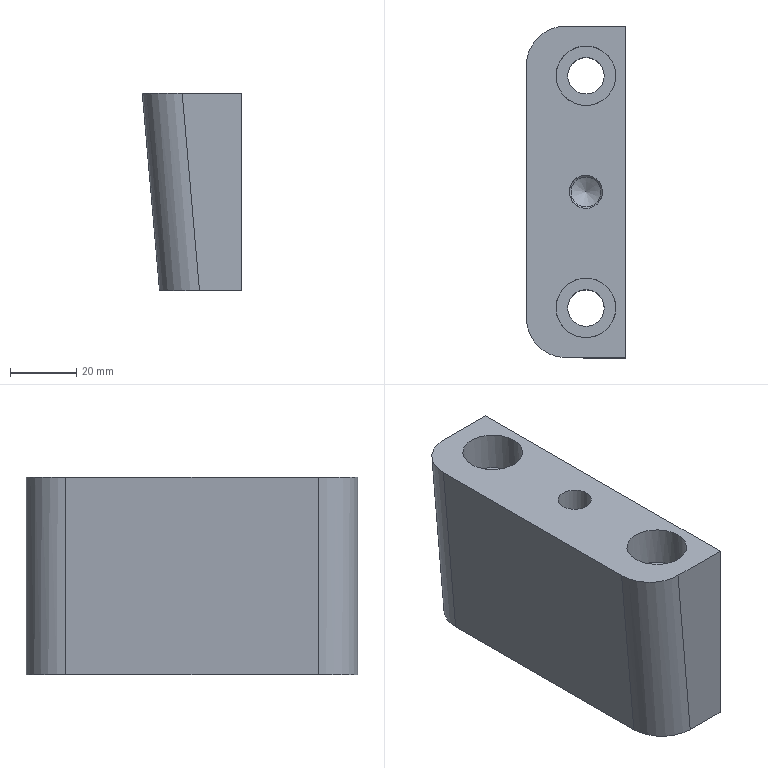Part | STEP file | solid 131 | 1 solid | 18 faces | box 30 x 100 x 59.496 mm | volume 142436 mm3 | plane 8 | cylinder 8 | cone 2 | commonest cylinder face diameters 11 x2 18 x2 24 x2 9 x1 10 x1